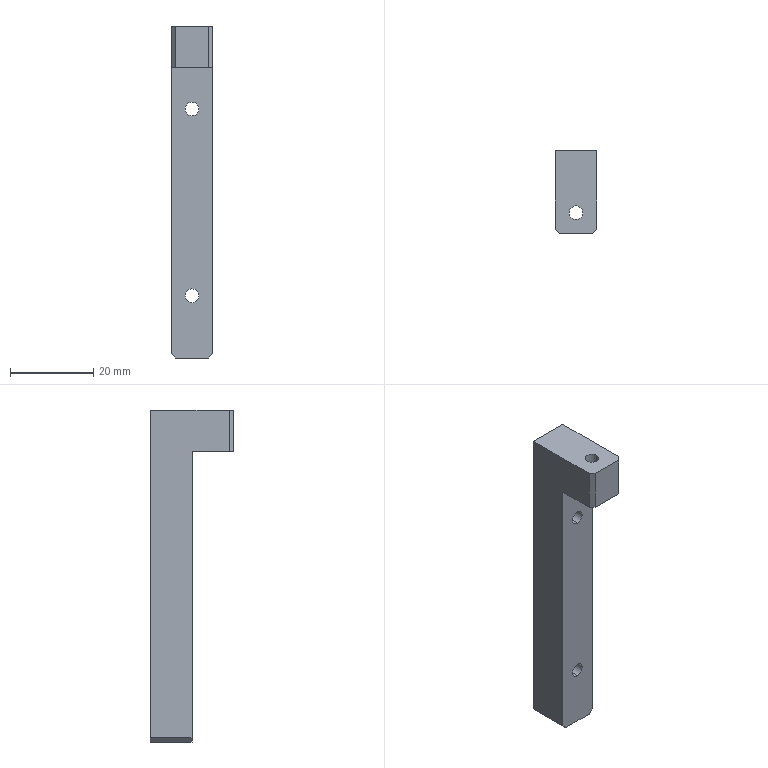Part | SolidWorks | features HoleWzd 2, Chamfer 1, Extrusion 1, ICE 1 | 1 solid | 18 faces | box 10 x 20 x 80 mm | volume 8723 mm3 | plane 12 | cylinder 6 | commonest cylinder face diameters 3.3 x6
STEP:
#1=CARTESIAN_POINT('',(5.,0.,-26.65));
#2=VERTEX_POINT('',#1);
#3=CARTESIAN_POINT('',(5.,0.,-23.35));
#4=VERTEX_POINT('',#3);
#5=CARTESIAN_POINT('',(5.,0.,-25.));
#6=DIRECTION('',(0.,1.,0.));
#7=DIRECTION('',(0.,0.,1.));
#8=AXIS2_PLACEMENT_3D('',#5,#6,#7);
#9=CIRCLE('',#8,1.65);
#10=EDGE_CURVE('',#2,#4,#9,.T.);
#11=ORIENTED_EDGE('',*,*,#10,.F.);
#12=CARTESIAN_POINT('',(5.,10.,-26.65));
#13=VERTEX_POINT('',#12);
#14=CARTESIAN_POINT('',(5.,10.,-26.65));
#15=DIRECTION('',(0.,1.,0.));
#16=VECTOR('',#15,1000.);
#17=LINE('',#14,#16);
#18=EDGE_CURVE('',#2,#13,#17,.T.);
#19=ORIENTED_EDGE('',*,*,#18,.T.);
#20=CARTESIAN_POINT('',(5.,10.,-23.35));
#21=VERTEX_POINT('',#20);
#22=CARTESIAN_POINT('',(5.,10.,-25.));
#23=DIRECTION('',(0.,1.,0.));
#24=DIRECTION('',(0.,0.,1.));
#25=AXIS2_PLACEMENT_3D('',#22,#23,#24);
#26=CIRCLE('',#25,1.65);
#27=EDGE_CURVE('',#13,#21,#26,.T.);
#28=ORIENTED_EDGE('',*,*,#27,.T.);
#29=CARTESIAN_POINT('',(5.,10.,-23.35));
#30=DIRECTION('',(0.,1.,0.));
#31=VECTOR('',#30,1000.);
#32=LINE('',#29,#31);
#33=EDGE_CURVE('',#4,#21,#32,.T.);
#34=ORIENTED_EDGE('',*,*,#33,.F.);
#35=EDGE_LOOP('',(#11,#19,#28,#34));
#36=FACE_OUTER_BOUND('',#35,.T.);
#37=CARTESIAN_POINT('',(5.,10.,-25.));
#38=DIRECTION('',(0.,1.,0.));
#39=DIRECTION('',(0.,0.,1.));
#40=AXIS2_PLACEMENT_3D('',#37,#38,#39);
#41=CYLINDRICAL_SURFACE('',#40,1.65);
#42=ADVANCED_FACE('',(#36),#41,.F.);
#43=CARTESIAN_POINT('',(5.,0.,18.35));
#44=VERTEX_POINT('',#43);
#45=CARTESIAN_POINT('',(5.,0.,21.65));
#46=VERTEX_POINT('',#45);
#47=CARTESIAN_POINT('',(5.,0.,20.));
#48=DIRECTION('',(0.,1.,0.));
#49=DIRECTION('',(0.,0.,1.));
#50=AXIS2_PLACEMENT_3D('',#47,#48,#49);
#51=CIRCLE('',#50,1.65);
#52=EDGE_CURVE('',#44,#46,#51,.T.);
#53=ORIENTED_EDGE('',*,*,#52,.F.);
#54=CARTESIAN_POINT('',(5.,10.,18.35));
#55=VERTEX_POINT('',#54);
#56=CARTESIAN_POINT('',(5.,10.,18.35));
#57=DIRECTION('',(0.,1.,0.));
#58=VECTOR('',#57,1000.);
#59=LINE('',#56,#58);
#60=EDGE_CURVE('',#44,#55,#59,.T.);
#61=ORIENTED_EDGE('',*,*,#60,.T.);
#62=CARTESIAN_POINT('',(5.,10.,21.65));
#63=VERTEX_POINT('',#62);
#64=CARTESIAN_POINT('',(5.,10.,20.));
#65=DIRECTION('',(0.,1.,0.));
#66=DIRECTION('',(0.,0.,1.));
#67=AXIS2_PLACEMENT_3D('',#64,#65,#66);
#68=CIRCLE('',#67,1.65);
#69=EDGE_CURVE('',#55,#63,#68,.T.);
#70=ORIENTED_EDGE('',*,*,#69,.T.);
#71=CARTESIAN_POINT('',(5.,10.,21.65));
#72=DIRECTION('',(0.,1.,0.));
#73=VECTOR('',#72,1000.);
#74=LINE('',#71,#73);
#75=EDGE_CURVE('',#46,#63,#74,.T.);
#76=ORIENTED_EDGE('',*,*,#75,.F.);
#77=EDGE_LOOP('',(#53,#61,#70,#76));
#78=FACE_OUTER_BOUND('',#77,.T.);
#79=CARTESIAN_POINT('',(5.,10.,20.));
#80=DIRECTION('',(0.,1.,0.));
#81=DIRECTION('',(0.,0.,1.));
#82=AXIS2_PLACEMENT_3D('',#79,#80,#81);
#83=CYLINDRICAL_SURFACE('',#82,1.65);
#84=ADVANCED_FACE('',(#78),#83,.F.);
#85=CARTESIAN_POINT('',(6.65,-5.,40.));
#86=VERTEX_POINT('',#85);
#87=CARTESIAN_POINT('',(3.35,-5.,40.));
#88=VERTEX_POINT('',#87);
#89=CARTESIAN_POINT('',(5.,-5.,40.));
#90=DIRECTION('',(0.,0.,-1.));
#91=DIRECTION('',(-1.,0.,0.));
#92=AXIS2_PLACEMENT_3D('',#89,#90,#91);
#93=CIRCLE('',#92,1.65);
#94=EDGE_CURVE('',#86,#88,#93,.T.);
#95=ORIENTED_EDGE('',*,*,#94,.F.);
#96=CARTESIAN_POINT('',(6.65,-5.,30.));
#97=VERTEX_POINT('',#96);
#98=CARTESIAN_POINT('',(6.65,-5.,30.));
#99=DIRECTION('',(0.,0.,-1.));
#100=VECTOR('',#99,1000.);
#101=LINE('',#98,#100);
#102=EDGE_CURVE('',#86,#97,#101,.T.);
#103=ORIENTED_EDGE('',*,*,#102,.T.);
#104=CARTESIAN_POINT('',(3.35,-5.,30.));
#105=VERTEX_POINT('',#104);
#106=CARTESIAN_POINT('',(5.,-5.,30.));
#107=DIRECTION('',(0.,0.,-1.));
#108=DIRECTION('',(-1.,0.,0.));
#109=AXIS2_PLACEMENT_3D('',#106,#107,#108);
#110=CIRCLE('',#109,1.65);
#111=EDGE_CURVE('',#97,#105,#110,.T.);
#112=ORIENTED_EDGE('',*,*,#111,.T.);
#113=CARTESIAN_POINT('',(3.35,-5.,30.));
#114=DIRECTION('',(0.,0.,-1.));
#115=VECTOR('',#114,1000.);
#116=LINE('',#113,#115);
#117=EDGE_CURVE('',#88,#105,#116,.T.);
#118=ORIENTED_EDGE('',*,*,#117,.F.);
#119=EDGE_LOOP('',(#95,#103,#112,#118));
#120=FACE_OUTER_BOUND('',#119,.T.);
#121=CARTESIAN_POINT('',(5.,-5.,30.));
#122=DIRECTION('',(0.,0.,-1.));
#123=DIRECTION('',(-1.,0.,0.));
#124=AXIS2_PLACEMENT_3D('',#121,#122,#123);
#125=CYLINDRICAL_SURFACE('',#124,1.65);
#126=ADVANCED_FACE('',(#120),#125,.F.);
#127=CARTESIAN_POINT('',(9.,0.,-40.));
#128=VERTEX_POINT('',#127);
#129=CARTESIAN_POINT('',(1.,0.,-40.));
#130=VERTEX_POINT('',#129);
#131=CARTESIAN_POINT('',(10.,0.,-40.));
#132=DIRECTION('',(-1.,0.,0.));
#133=VECTOR('',#132,1000.);
#134=LINE('',#131,#133);
#135=EDGE_CURVE('',#128,#130,#134,.T.);
#136=ORIENTED_EDGE('',*,*,#135,.T.);
#137=CARTESIAN_POINT('',(1.,10.,-40.));
#138=VERTEX_POINT('',#137);
#139=CARTESIAN_POINT('',(1.,10.,-40.));
#140=DIRECTION('',(0.,1.,0.));
#141=VECTOR('',#140,1000.);
#142=LINE('',#139,#141);
#143=EDGE_CURVE('',#130,#138,#142,.T.);
#144=ORIENTED_EDGE('',*,*,#143,.T.);
#145=CARTESIAN_POINT('',(9.,10.,-40.));
#146=VERTEX_POINT('',#145);
#147=CARTESIAN_POINT('',(10.,10.,-40.));
#148=DIRECTION('',(-1.,0.,0.));
#149=VECTOR('',#148,1000.);
#150=LINE('',#147,#149);
#151=EDGE_CURVE('',#146,#138,#150,.T.);
#152=ORIENTED_EDGE('',*,*,#151,.F.);
#153=CARTESIAN_POINT('',(9.,-10.,-40.));
#154=DIRECTION('',(0.,-1.,0.));
#155=VECTOR('',#154,1000.);
#156=LINE('',#153,#155);
#157=EDGE_CURVE('',#146,#128,#156,.T.);
#158=ORIENTED_EDGE('',*,*,#157,.T.);
#159=EDGE_LOOP('',(#136,#144,#152,#158));
#160=FACE_OUTER_BOUND('',#159,.T.);
#161=CARTESIAN_POINT('',(10.,-10.,-40.));
#162=DIRECTION('',(0.,0.,1.));
#163=DIRECTION('',(1.,0.,0.));
#164=AXIS2_PLACEMENT_3D('',#161,#162,#163);
#165=PLANE('',#164);
#166=ADVANCED_FACE('',(#160),#165,.F.);
#167=CARTESIAN_POINT('',(5.,10.,-25.));
#168=DIRECTION('',(0.,1.,0.));
#169=DIRECTION('',(0.,0.,1.));
#170=AXIS2_PLACEMENT_3D('',#167,#168,#169);
#171=CIRCLE('',#170,1.65);
#172=EDGE_CURVE('',#21,#13,#171,.T.);
#173=ORIENTED_EDGE('',*,*,#172,.F.);
#174=ORIENTED_EDGE('',*,*,#27,.F.);
#175=EDGE_LOOP('',(#173,#174));
#176=FACE_BOUND('',#175,.T.);
#177=CARTESIAN_POINT('',(5.,10.,20.));
#178=DIRECTION('',(0.,1.,0.));
#179=DIRECTION('',(0.,0.,1.));
#180=AXIS2_PLACEMENT_3D('',#177,#178,#179);
#181=CIRCLE('',#180,1.65);
#182=EDGE_CURVE('',#63,#55,#181,.T.);
#183=ORIENTED_EDGE('',*,*,#182,.F.);
#184=ORIENTED_EDGE('',*,*,#69,.F.);
#185=EDGE_LOOP('',(#183,#184));
#186=FACE_BOUND('',#185,.T.);
#187=ORIENTED_EDGE('',*,*,#151,.T.);
#188=CARTESIAN_POINT('',(0.,10.,-39.));
#189=VERTEX_POINT('',#188);
#190=CARTESIAN_POINT('',(1.,10.,-40.));
#191=DIRECTION('',(-0.7071,0.,0.7071));
#192=VECTOR('',#191,1000.);
#193=LINE('',#190,#192);
#194=EDGE_CURVE('',#138,#189,#193,.T.);
#195=ORIENTED_EDGE('',*,*,#194,.T.);
#196=CARTESIAN_POINT('',(0.,10.,40.));
#197=VERTEX_POINT('',#196);
#198=CARTESIAN_POINT('',(0.,10.,40.));
#199=DIRECTION('',(0.,0.,1.));
#200=VECTOR('',#199,1000.);
#201=LINE('',#198,#200);
#202=EDGE_CURVE('',#189,#197,#201,.T.);
#203=ORIENTED_EDGE('',*,*,#202,.T.);
#204=CARTESIAN_POINT('',(10.,10.,40.));
#205=VERTEX_POINT('',#204);
#206=CARTESIAN_POINT('',(10.,10.,40.));
#207=DIRECTION('',(-1.,0.,0.));
#208=VECTOR('',#207,1000.);
#209=LINE('',#206,#208);
#210=EDGE_CURVE('',#205,#197,#209,.T.);
#211=ORIENTED_EDGE('',*,*,#210,.F.);
#212=CARTESIAN_POINT('',(10.,10.,-39.));
#213=VERTEX_POINT('',#212);
#214=CARTESIAN_POINT('',(10.,10.,40.));
#215=DIRECTION('',(0.,0.,1.));
#216=VECTOR('',#215,1000.);
#217=LINE('',#214,#216);
#218=EDGE_CURVE('',#213,#205,#217,.T.);
#219=ORIENTED_EDGE('',*,*,#218,.F.);
#220=CARTESIAN_POINT('',(10.,10.,-39.));
#221=DIRECTION('',(-0.7071,0.,-0.7071));
#222=VECTOR('',#221,1000.);
#223=LINE('',#220,#222);
#224=EDGE_CURVE('',#213,#146,#223,.T.);
#225=ORIENTED_EDGE('',*,*,#224,.T.);
#226=EDGE_LOOP('',(#187,#195,#203,#211,#219,#225));
#227=FACE_OUTER_BOUND('',#226,.T.);
#228=CARTESIAN_POINT('',(10.,10.,40.));
#229=DIRECTION('',(0.,-1.,0.));
#230=DIRECTION('',(0.,0.,-1.));
#231=AXIS2_PLACEMENT_3D('',#228,#229,#230);
#232=PLANE('',#231);
#233=ADVANCED_FACE('',(#176,#186,#227),#232,.F.);
#234=CARTESIAN_POINT('',(5.,-5.,40.));
#235=DIRECTION('',(0.,0.,-1.));
#236=DIRECTION('',(-1.,0.,0.));
#237=AXIS2_PLACEMENT_3D('',#234,#235,#236);
#238=CIRCLE('',#237,1.65);
#239=EDGE_CURVE('',#88,#86,#238,.T.);
#240=ORIENTED_EDGE('',*,*,#239,.T.);
#241=ORIENTED_EDGE('',*,*,#94,.T.);
#242=EDGE_LOOP('',(#240,#241));
#243=FACE_BOUND('',#242,.T.);
#244=CARTESIAN_POINT('',(9.,-10.,40.));
#245=VERTEX_POINT('',#244);
#246=CARTESIAN_POINT('',(1.,-10.,40.));
#247=VERTEX_POINT('',#246);
#248=CARTESIAN_POINT('',(10.,-10.,40.));
#249=DIRECTION('',(-1.,0.,0.));
#250=VECTOR('',#249,1000.);
#251=LINE('',#248,#250);
#252=EDGE_CURVE('',#245,#247,#251,.T.);
#253=ORIENTED_EDGE('',*,*,#252,.F.);
#254=CARTESIAN_POINT('',(10.,-9.,40.));
#255=VERTEX_POINT('',#254);
#256=CARTESIAN_POINT('',(10.,-9.,40.));
#257=DIRECTION('',(0.7071,0.7071,0.));
#258=VECTOR('',#257,1000.);
#259=LINE('',#256,#258);
#260=EDGE_CURVE('',#245,#255,#259,.T.);
#261=ORIENTED_EDGE('',*,*,#260,.T.);
#262=CARTESIAN_POINT('',(10.,-10.,40.));
#263=DIRECTION('',(0.,-1.,0.));
#264=VECTOR('',#263,1000.);
#265=LINE('',#262,#264);
#266=EDGE_CURVE('',#205,#255,#265,.T.);
#267=ORIENTED_EDGE('',*,*,#266,.F.);
#268=ORIENTED_EDGE('',*,*,#210,.T.);
#269=CARTESIAN_POINT('',(0.,-9.,40.));
#270=VERTEX_POINT('',#269);
#271=CARTESIAN_POINT('',(0.,-10.,40.));
#272=DIRECTION('',(0.,-1.,0.));
#273=VECTOR('',#272,1000.);
#274=LINE('',#271,#273);
#275=EDGE_CURVE('',#197,#270,#274,.T.);
#276=ORIENTED_EDGE('',*,*,#275,.T.);
#277=CARTESIAN_POINT('',(1.,-10.,40.));
#278=DIRECTION('',(0.7071,-0.7071,0.));
#279=VECTOR('',#278,1000.);
#280=LINE('',#277,#279);
#281=EDGE_CURVE('',#270,#247,#280,.T.);
#282=ORIENTED_EDGE('',*,*,#281,.T.);
#283=EDGE_LOOP('',(#253,#261,#267,#268,#276,#282));
#284=FACE_OUTER_BOUND('',#283,.T.);
#285=CARTESIAN_POINT('',(10.,-10.,40.));
#286=DIRECTION('',(0.,0.,-1.));
#287=DIRECTION('',(-1.,0.,0.));
#288=AXIS2_PLACEMENT_3D('',#285,#286,#287);
#289=PLANE('',#288);
#290=ADVANCED_FACE('',(#243,#284),#289,.F.);
#291=CARTESIAN_POINT('',(9.,-10.,30.));
#292=VERTEX_POINT('',#291);
#293=CARTESIAN_POINT('',(1.,-10.,30.));
#294=VERTEX_POINT('',#293);
#295=CARTESIAN_POINT('',(10.,-10.,30.));
#296=DIRECTION('',(-1.,0.,0.));
#297=VECTOR('',#296,1000.);
#298=LINE('',#295,#297);
#299=EDGE_CURVE('',#292,#294,#298,.T.);
#300=ORIENTED_EDGE('',*,*,#299,.F.);
#301=CARTESIAN_POINT('',(9.,-10.,40.));
#302=DIRECTION('',(0.,0.,1.));
#303=VECTOR('',#302,1000.);
#304=LINE('',#301,#303);
#305=EDGE_CURVE('',#292,#245,#304,.T.);
#306=ORIENTED_EDGE('',*,*,#305,.T.);
#307=ORIENTED_EDGE('',*,*,#252,.T.);
#308=CARTESIAN_POINT('',(1.,-10.,30.));
#309=DIRECTION('',(0.,0.,-1.));
#310=VECTOR('',#309,1000.);
#311=LINE('',#308,#310);
#312=EDGE_CURVE('',#247,#294,#311,.T.);
#313=ORIENTED_EDGE('',*,*,#312,.T.);
#314=EDGE_LOOP('',(#300,#306,#307,#313));
#315=FACE_OUTER_BOUND('',#314,.T.);
#316=CARTESIAN_POINT('',(10.,-10.,40.));
#317=DIRECTION('',(0.,1.,0.));
#318=DIRECTION('',(0.,0.,1.));
#319=AXIS2_PLACEMENT_3D('',#316,#317,#318);
#320=PLANE('',#319);
#321=ADVANCED_FACE('',(#315),#320,.F.);
#322=CARTESIAN_POINT('',(10.,0.,30.));
#323=VERTEX_POINT('',#322);
#324=CARTESIAN_POINT('',(10.,0.,-39.));
#325=VERTEX_POINT('',#324);
#326=CARTESIAN_POINT('',(10.,0.,-40.));
#327=DIRECTION('',(0.,0.,-1.));
#328=VECTOR('',#327,1000.);
#329=LINE('',#326,#328);
#330=EDGE_CURVE('',#323,#325,#329,.T.);
#331=ORIENTED_EDGE('',*,*,#330,.T.);
#332=CARTESIAN_POINT('',(10.,0.,-39.));
#333=DIRECTION('',(0.,1.,0.));
#334=VECTOR('',#333,1000.);
#335=LINE('',#332,#334);
#336=EDGE_CURVE('',#325,#213,#335,.T.);
#337=ORIENTED_EDGE('',*,*,#336,.T.);
#338=ORIENTED_EDGE('',*,*,#218,.T.);
#339=ORIENTED_EDGE('',*,*,#266,.T.);
#340=CARTESIAN_POINT('',(10.,-9.,30.));
#341=VERTEX_POINT('',#340);
#342=CARTESIAN_POINT('',(10.,-9.,0.));
#343=DIRECTION('',(0.,0.,-1.));
#344=VECTOR('',#343,1000.);
#345=LINE('',#342,#344);
#346=EDGE_CURVE('',#255,#341,#345,.T.);
#347=ORIENTED_EDGE('',*,*,#346,.T.);
#348=CARTESIAN_POINT('',(10.,-10.,30.));
#349=DIRECTION('',(0.,1.,0.));
#350=VECTOR('',#349,1000.);
#351=LINE('',#348,#350);
#352=EDGE_CURVE('',#341,#323,#351,.T.);
#353=ORIENTED_EDGE('',*,*,#352,.T.);
#354=EDGE_LOOP('',(#331,#337,#338,#339,#347,#353));
#355=FACE_OUTER_BOUND('',#354,.T.);
#356=CARTESIAN_POINT('',(10.,0.,0.));
#357=DIRECTION('',(-1.,0.,0.));
#358=DIRECTION('',(0.,0.,1.));
#359=AXIS2_PLACEMENT_3D('',#356,#357,#358);
#360=PLANE('',#359);
#361=ADVANCED_FACE('',(#355),#360,.F.);
#362=ORIENTED_EDGE('',*,*,#202,.F.);
#363=CARTESIAN_POINT('',(0.,0.,-39.));
#364=VERTEX_POINT('',#363);
#365=CARTESIAN_POINT('',(0.,0.,-39.));
#366=DIRECTION('',(0.,-1.,0.));
#367=VECTOR('',#366,1000.);
#368=LINE('',#365,#367);
#369=EDGE_CURVE('',#189,#364,#368,.T.);
#370=ORIENTED_EDGE('',*,*,#369,.T.);
#371=CARTESIAN_POINT('',(0.,0.,30.));
#372=VERTEX_POINT('',#371);
#373=CARTESIAN_POINT('',(0.,0.,-40.));
#374=DIRECTION('',(0.,0.,-1.));
#375=VECTOR('',#374,1000.);
#376=LINE('',#373,#375);
#377=EDGE_CURVE('',#372,#364,#376,.T.);
#378=ORIENTED_EDGE('',*,*,#377,.F.);
#379=CARTESIAN_POINT('',(0.,-9.,30.));
#380=VERTEX_POINT('',#379);
#381=CARTESIAN_POINT('',(0.,-10.,30.));
#382=DIRECTION('',(0.,1.,0.));
#383=VECTOR('',#382,1000.);
#384=LINE('',#381,#383);
#385=EDGE_CURVE('',#380,#372,#384,.T.);
#386=ORIENTED_EDGE('',*,*,#385,.F.);
#387=CARTESIAN_POINT('',(0.,-9.,40.));
#388=DIRECTION('',(0.,0.,1.));
#389=VECTOR('',#388,1000.);
#390=LINE('',#387,#389);
#391=EDGE_CURVE('',#380,#270,#390,.T.);
#392=ORIENTED_EDGE('',*,*,#391,.T.);
#393=ORIENTED_EDGE('',*,*,#275,.F.);
#394=EDGE_LOOP('',(#362,#370,#378,#386,#392,#393));
#395=FACE_OUTER_BOUND('',#394,.T.);
#396=CARTESIAN_POINT('',(0.,0.,0.));
#397=DIRECTION('',(-1.,0.,0.));
#398=DIRECTION('',(0.,0.,1.));
#399=AXIS2_PLACEMENT_3D('',#396,#397,#398);
#400=PLANE('',#399);
#401=ADVANCED_FACE('',(#395),#400,.T.);
#402=CARTESIAN_POINT('',(5.,0.,-25.));
#403=DIRECTION('',(0.,1.,0.));
#404=DIRECTION('',(0.,0.,1.));
#405=AXIS2_PLACEMENT_3D('',#402,#403,#404);
#406=CIRCLE('',#405,1.65);
#407=EDGE_CURVE('',#4,#2,#406,.T.);
#408=ORIENTED_EDGE('',*,*,#407,.T.);
#409=ORIENTED_EDGE('',*,*,#10,.T.);
#410=EDGE_LOOP('',(#408,#409));
#411=FACE_BOUND('',#410,.T.);
#412=CARTESIAN_POINT('',(5.,0.,20.));
#413=DIRECTION('',(0.,1.,0.));
#414=DIRECTION('',(0.,0.,1.));
#415=AXIS2_PLACEMENT_3D('',#412,#413,#414);
#416=CIRCLE('',#415,1.65);
#417=EDGE_CURVE('',#46,#44,#416,.T.);
#418=ORIENTED_EDGE('',*,*,#417,.T.);
#419=ORIENTED_EDGE('',*,*,#52,.T.);
#420=EDGE_LOOP('',(#418,#419));
#421=FACE_BOUND('',#420,.T.);
#422=ORIENTED_EDGE('',*,*,#377,.T.);
#423=CARTESIAN_POINT('',(1.,0.,-40.));
#424=DIRECTION('',(0.7071,0.,-0.7071));
#425=VECTOR('',#424,1000.);
#426=LINE('',#423,#425);
#427=EDGE_CURVE('',#364,#130,#426,.T.);
#428=ORIENTED_EDGE('',*,*,#427,.T.);
#429=ORIENTED_EDGE('',*,*,#135,.F.);
#430=CARTESIAN_POINT('',(10.,0.,-39.));
#431=DIRECTION('',(0.7071,0.,0.7071));
#432=VECTOR('',#431,1000.);
#433=LINE('',#430,#432);
#434=EDGE_CURVE('',#128,#325,#433,.T.);
#435=ORIENTED_EDGE('',*,*,#434,.T.);
#436=ORIENTED_EDGE('',*,*,#330,.F.);
#437=CARTESIAN_POINT('',(10.,0.,30.));
#438=DIRECTION('',(-1.,0.,0.));
#439=VECTOR('',#438,1000.);
#440=LINE('',#437,#439);
#441=EDGE_CURVE('',#323,#372,#440,.T.);
#442=ORIENTED_EDGE('',*,*,#441,.T.);
#443=EDGE_LOOP('',(#422,#428,#429,#435,#436,#442));
#444=FACE_OUTER_BOUND('',#443,.T.);
#445=CARTESIAN_POINT('',(10.,0.,-40.));
#446=DIRECTION('',(0.,1.,0.));
#447=DIRECTION('',(0.,0.,1.));
#448=AXIS2_PLACEMENT_3D('',#445,#446,#447);
#449=PLANE('',#448);
#450=ADVANCED_FACE('',(#411,#421,#444),#449,.F.);
#451=CARTESIAN_POINT('',(5.,-5.,30.));
#452=DIRECTION('',(0.,0.,-1.));
#453=DIRECTION('',(-1.,0.,0.));
#454=AXIS2_PLACEMENT_3D('',#451,#452,#453);
#455=CIRCLE('',#454,1.65);
#456=EDGE_CURVE('',#105,#97,#455,.T.);
#457=ORIENTED_EDGE('',*,*,#456,.F.);
#458=ORIENTED_EDGE('',*,*,#111,.F.);
#459=EDGE_LOOP('',(#457,#458));
#460=FACE_BOUND('',#459,.T.);
#461=ORIENTED_EDGE('',*,*,#352,.F.);
#462=CARTESIAN_POINT('',(10.,-9.,30.));
#463=DIRECTION('',(-0.7071,-0.7071,0.));
#464=VECTOR('',#463,1000.);
#465=LINE('',#462,#464);
#466=EDGE_CURVE('',#341,#292,#465,.T.);
#467=ORIENTED_EDGE('',*,*,#466,.T.);
#468=ORIENTED_EDGE('',*,*,#299,.T.);
#469=CARTESIAN_POINT('',(1.,-10.,30.));
#470=DIRECTION('',(-0.7071,0.7071,0.));
#471=VECTOR('',#470,1000.);
#472=LINE('',#469,#471);
#473=EDGE_CURVE('',#294,#380,#472,.T.);
#474=ORIENTED_EDGE('',*,*,#473,.T.);
#475=ORIENTED_EDGE('',*,*,#385,.T.);
#476=ORIENTED_EDGE('',*,*,#441,.F.);
#477=EDGE_LOOP('',(#461,#467,#468,#474,#475,#476));
#478=FACE_OUTER_BOUND('',#477,.T.);
#479=CARTESIAN_POINT('',(10.,-10.,30.));
#480=DIRECTION('',(0.,0.,1.));
#481=DIRECTION('',(1.,0.,0.));
#482=AXIS2_PLACEMENT_3D('',#479,#480,#481);
#483=PLANE('',#482);
#484=ADVANCED_FACE('',(#460,#478),#483,.F.);
#485=ORIENTED_EDGE('',*,*,#102,.F.);
#486=ORIENTED_EDGE('',*,*,#239,.F.);
#487=ORIENTED_EDGE('',*,*,#117,.T.);
#488=ORIENTED_EDGE('',*,*,#456,.T.);
#489=EDGE_LOOP('',(#485,#486,#487,#488));
#490=FACE_OUTER_BOUND('',#489,.T.);
#491=CARTESIAN_POINT('',(5.,-5.,30.));
#492=DIRECTION('',(0.,0.,-1.));
#493=DIRECTION('',(-1.,0.,0.));
#494=AXIS2_PLACEMENT_3D('',#491,#492,#493);
#495=CYLINDRICAL_SURFACE('',#494,1.65);
#496=ADVANCED_FACE('',(#490),#495,.F.);
#497=ORIENTED_EDGE('',*,*,#427,.F.);
#498=ORIENTED_EDGE('',*,*,#369,.F.);
#499=ORIENTED_EDGE('',*,*,#194,.F.);
#500=ORIENTED_EDGE('',*,*,#143,.F.);
#501=EDGE_LOOP('',(#497,#498,#499,#500));
#502=FACE_OUTER_BOUND('',#501,.T.);
#503=CARTESIAN_POINT('',(1.,-10.,-40.));
#504=DIRECTION('',(-0.7071,0.,-0.7071));
#505=DIRECTION('',(0.,-1.,0.));
#506=AXIS2_PLACEMENT_3D('',#503,#504,#505);
#507=PLANE('',#506);
#508=ADVANCED_FACE('',(#502),#507,.T.);
#509=ORIENTED_EDGE('',*,*,#434,.F.);
#510=ORIENTED_EDGE('',*,*,#157,.F.);
#511=ORIENTED_EDGE('',*,*,#224,.F.);
#512=ORIENTED_EDGE('',*,*,#336,.F.);
#513=EDGE_LOOP('',(#509,#510,#511,#512));
#514=FACE_OUTER_BOUND('',#513,.T.);
#515=CARTESIAN_POINT('',(10.,0.,-39.));
#516=DIRECTION('',(-0.7071,0.,0.7071));
#517=DIRECTION('',(0.,1.,0.));
#518=AXIS2_PLACEMENT_3D('',#515,#516,#517);
#519=PLANE('',#518);
#520=ADVANCED_FACE('',(#514),#519,.F.);
#521=ORIENTED_EDGE('',*,*,#260,.F.);
#522=ORIENTED_EDGE('',*,*,#305,.F.);
#523=ORIENTED_EDGE('',*,*,#466,.F.);
#524=ORIENTED_EDGE('',*,*,#346,.F.);
#525=EDGE_LOOP('',(#521,#522,#523,#524));
#526=FACE_OUTER_BOUND('',#525,.T.);
#527=CARTESIAN_POINT('',(10.,-9.,0.));
#528=DIRECTION('',(-0.7071,0.7071,0.));
#529=DIRECTION('',(0.,0.,-1.));
#530=AXIS2_PLACEMENT_3D('',#527,#528,#529);
#531=PLANE('',#530);
#532=ADVANCED_FACE('',(#526),#531,.F.);
#533=ORIENTED_EDGE('',*,*,#281,.F.);
#534=ORIENTED_EDGE('',*,*,#391,.F.);
#535=ORIENTED_EDGE('',*,*,#473,.F.);
#536=ORIENTED_EDGE('',*,*,#312,.F.);
#537=EDGE_LOOP('',(#533,#534,#535,#536));
#538=FACE_OUTER_BOUND('',#537,.T.);
#539=CARTESIAN_POINT('',(1.,-10.,40.));
#540=DIRECTION('',(-0.7071,-0.7071,0.));
#541=DIRECTION('',(0.,0.,1.));
#542=AXIS2_PLACEMENT_3D('',#539,#540,#541);
#543=PLANE('',#542);
#544=ADVANCED_FACE('',(#538),#543,.T.);
#545=ORIENTED_EDGE('',*,*,#60,.F.);
#546=ORIENTED_EDGE('',*,*,#417,.F.);
#547=ORIENTED_EDGE('',*,*,#75,.T.);
#548=ORIENTED_EDGE('',*,*,#182,.T.);
#549=EDGE_LOOP('',(#545,#546,#547,#548));
#550=FACE_OUTER_BOUND('',#549,.T.);
#551=CARTESIAN_POINT('',(5.,10.,20.));
#552=DIRECTION('',(0.,1.,0.));
#553=DIRECTION('',(0.,0.,1.));
#554=AXIS2_PLACEMENT_3D('',#551,#552,#553);
#555=CYLINDRICAL_SURFACE('',#554,1.65);
#556=ADVANCED_FACE('',(#550),#555,.F.);
#557=ORIENTED_EDGE('',*,*,#18,.F.);
#558=ORIENTED_EDGE('',*,*,#407,.F.);
#559=ORIENTED_EDGE('',*,*,#33,.T.);
#560=ORIENTED_EDGE('',*,*,#172,.T.);
#561=EDGE_LOOP('',(#557,#558,#559,#560));
#562=FACE_OUTER_BOUND('',#561,.T.);
#563=CARTESIAN_POINT('',(5.,10.,-25.));
#564=DIRECTION('',(0.,1.,0.));
#565=DIRECTION('',(0.,0.,1.));
#566=AXIS2_PLACEMENT_3D('',#563,#564,#565);
#567=CYLINDRICAL_SURFACE('',#566,1.65);
#568=ADVANCED_FACE('',(#562),#567,.F.);
#569=CLOSED_SHELL('',(#42,#84,#126,#166,#233,#290,#321,#361,#401,#450,#484,#496,#508,#520,#532,#544,#556,#568));
#570=MANIFOLD_SOLID_BREP('',#569);
#571=CARTESIAN_POINT('',(0.,0.,0.));
#572=DIRECTION('',(0.,0.,1.));
#573=DIRECTION('',(1.,0.,0.));
#574=AXIS2_PLACEMENT_3D('',#571,#572,#573);
#575=(LENGTH_UNIT()NAMED_UNIT(*)SI_UNIT(.MILLI.,.METRE.));
#576=UNCERTAINTY_MEASURE_WITH_UNIT(LENGTH_MEASURE(0.00001),#575,'','');
#577=(NAMED_UNIT(*)PLANE_ANGLE_UNIT()SI_UNIT($,.RADIAN.));
#578=(NAMED_UNIT(*)SI_UNIT($,.STERADIAN.)SOLID_ANGLE_UNIT());
#579=(GEOMETRIC_REPRESENTATION_CONTEXT(3)GLOBAL_UNCERTAINTY_ASSIGNED_CONTEXT((#576))GLOBAL_UNIT_ASSIGNED_CONTEXT((#575,#577,#578))REPRESENTATION_CONTEXT('',''));
#580=ADVANCED_BREP_SHAPE_REPRESENTATION('',(#570,#574),#579);